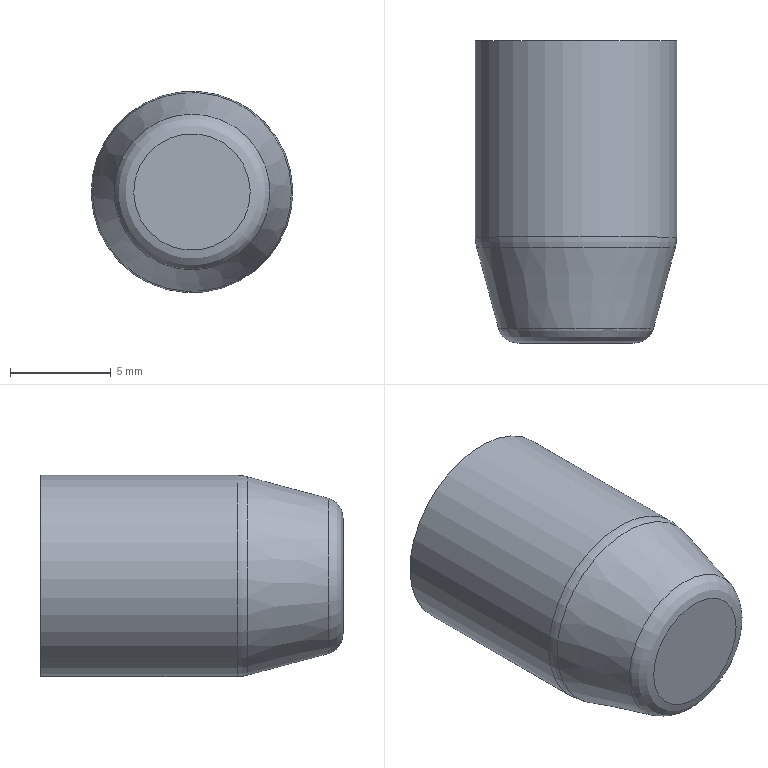Part | STEP file | 2_ESTAGIO_005 | 1 solid | 8 faces | box 10 x 15 x 10 mm | volume 994.545 mm3 | cone 2 | plane 2 | cylinder 2 | torus 2 | commonest cylinder face diameters 3.242 x1 10 x1
STEP:
#1=CARTESIAN_POINT('',(0.,0.,0.));
#2=DIRECTION('',(0.,0.,1.));
#3=DIRECTION('',(1.,0.,0.));
#4=AXIS2_PLACEMENT_3D('',#1,#2,#3);
#5=CARTESIAN_POINT('',(389.762,-538.65,378.626));
#6=VERTEX_POINT('',#5);
#7=CARTESIAN_POINT('',(388.339,-538.65,377.849));
#8=DIRECTION('',(0.,1.,0.));
#9=DIRECTION('',(1.,0.,0.));
#10=AXIS2_PLACEMENT_3D('',#7,#8,#9);
#11=CIRCLE('',#10,1.621);
#12=CARTESIAN_POINT('',(388.339,-539.009,377.849));
#13=DIRECTION('',(0.,1.,0.));
#14=DIRECTION('',(0.8776,0.,0.4794));
#15=AXIS2_PLACEMENT_3D('',#12,#13,#14);
#16=CONICAL_SURFACE('',#15,1.,1.047);
#17=CARTESIAN_POINT('',(-5.783,0.3585));
#18=DIRECTION('',(1.,0.));
#19=VECTOR('',#18,1.);
#20=LINE('',#17,#19);
#21=(GEOMETRIC_REPRESENTATION_CONTEXT(2)PARAMETRIC_REPRESENTATION_CONTEXT()REPRESENTATION_CONTEXT('',''));
#22=DEFINITIONAL_REPRESENTATION('',(#20),#21);
#23=PCURVE('',#16,#22);
#24=CARTESIAN_POINT('',(388.339,-528.75,377.849));
#25=DIRECTION('',(0.,-1.,0.));
#26=DIRECTION('',(0.8776,0.,0.4794));
#27=AXIS2_PLACEMENT_3D('',#24,#25,#26);
#28=CYLINDRICAL_SURFACE('',#27,1.621);
#29=CARTESIAN_POINT('',(12.066,9.9));
#30=DIRECTION('',(-1.,0.));
#31=VECTOR('',#30,1.);
#32=LINE('',#29,#31);
#33=(GEOMETRIC_REPRESENTATION_CONTEXT(2)PARAMETRIC_REPRESENTATION_CONTEXT()REPRESENTATION_CONTEXT('',''));
#34=DEFINITIONAL_REPRESENTATION('',(#32),#33);
#35=PCURVE('',#28,#34);
#36=SURFACE_CURVE('',#11,(#23,#35),.PCURVE_S1.);
#37=EDGE_CURVE('',#6,#6,#36,.T.);
#38=ORIENTED_EDGE('',*,*,#37,.F.);
#39=CARTESIAN_POINT('',(388.339,-539.586,377.849));
#40=VERTEX_POINT('',#39);
#41=CARTESIAN_POINT('',(388.339,-539.586,377.849));
#42=CARTESIAN_POINT('',(389.762,-538.65,378.626));
#43=B_SPLINE_CURVE_WITH_KNOTS('',1,(#41,#42),.UNSPECIFIED.,.F.,.F.,(2,2),(-1.155,0.7171),.PIECEWISE_BEZIER_KNOTS.);
#44=CARTESIAN_POINT('',(0.,0.));
#45=DIRECTION('',(0.,1.));
#46=VECTOR('',#45,1.);
#47=LINE('',#44,#46);
#48=(GEOMETRIC_REPRESENTATION_CONTEXT(2)PARAMETRIC_REPRESENTATION_CONTEXT()REPRESENTATION_CONTEXT('',''));
#49=DEFINITIONAL_REPRESENTATION('',(#47),#48);
#50=PCURVE('',#16,#49);
#51=CARTESIAN_POINT('',(6.283,0.));
#52=DIRECTION('',(0.,1.));
#53=VECTOR('',#52,1.);
#54=LINE('',#51,#53);
#55=(GEOMETRIC_REPRESENTATION_CONTEXT(2)PARAMETRIC_REPRESENTATION_CONTEXT()REPRESENTATION_CONTEXT('',''));
#56=DEFINITIONAL_REPRESENTATION('',(#54),#55);
#57=PCURVE('',#16,#56);
#58=SEAM_CURVE('',#43,(#50,#57),.PCURVE_S1.);
#59=EDGE_CURVE('',#40,#6,#58,.T.);
#60=ORIENTED_EDGE('',*,*,#59,.F.);
#61=ORIENTED_EDGE('',*,*,#59,.T.);
#62=EDGE_LOOP('',(#38,#60,#61));
#63=FACE_BOUND('',#62,.F.);
#64=ADVANCED_FACE('',(#63),#16,.F.);
#65=CARTESIAN_POINT('',(384.538,-528.65,381.097));
#66=VERTEX_POINT('',#65);
#67=CARTESIAN_POINT('',(388.339,-528.65,377.849));
#68=DIRECTION('',(0.,1.,0.));
#69=DIRECTION('',(1.,0.,0.));
#70=AXIS2_PLACEMENT_3D('',#67,#68,#69);
#71=CIRCLE('',#70,5.);
#72=CARTESIAN_POINT('',(393.232,-528.65,376.821));
#73=DIRECTION('',(0.,1.,0.));
#74=DIRECTION('',(0.,0.,1.));
#75=AXIS2_PLACEMENT_3D('',#72,#73,#74);
#76=PLANE('',#75);
#77=CARTESIAN_POINT('',(1.028,-4.893));
#78=DIRECTION('',(0.,1.));
#79=AXIS2_PLACEMENT_2D('',#77,#78);
#80=CIRCLE('',#79,5.);
#81=(GEOMETRIC_REPRESENTATION_CONTEXT(2)PARAMETRIC_REPRESENTATION_CONTEXT()REPRESENTATION_CONTEXT('',''));
#82=DEFINITIONAL_REPRESENTATION('',(#80),#81);
#83=PCURVE('',#76,#82);
#84=CARTESIAN_POINT('',(388.339,-536.15,377.849));
#85=DIRECTION('',(0.,1.,0.));
#86=DIRECTION('',(0.7602,0.,-0.6496));
#87=AXIS2_PLACEMENT_3D('',#84,#85,#86);
#88=CYLINDRICAL_SURFACE('',#87,5.);
#89=CARTESIAN_POINT('',(-0.7071,7.5));
#90=DIRECTION('',(1.,0.));
#91=VECTOR('',#90,1.);
#92=LINE('',#89,#91);
#93=(GEOMETRIC_REPRESENTATION_CONTEXT(2)PARAMETRIC_REPRESENTATION_CONTEXT()REPRESENTATION_CONTEXT('',''));
#94=DEFINITIONAL_REPRESENTATION('',(#92),#93);
#95=PCURVE('',#88,#94);
#96=SURFACE_CURVE('',#71,(#83,#95),.PCURVE_S1.);
#97=EDGE_CURVE('',#66,#66,#96,.T.);
#98=ORIENTED_EDGE('',*,*,#97,.T.);
#99=EDGE_LOOP('',(#98));
#100=FACE_BOUND('',#99,.T.);
#101=CARTESIAN_POINT('',(389.762,-528.65,378.626));
#102=VERTEX_POINT('',#101);
#103=CARTESIAN_POINT('',(388.339,-528.65,377.849));
#104=DIRECTION('',(0.,1.,0.));
#105=DIRECTION('',(1.,0.,0.));
#106=AXIS2_PLACEMENT_3D('',#103,#104,#105);
#107=CIRCLE('',#106,1.621);
#108=CARTESIAN_POINT('',(1.028,-4.893));
#109=DIRECTION('',(0.,1.));
#110=AXIS2_PLACEMENT_2D('',#108,#109);
#111=CIRCLE('',#110,1.621);
#112=(GEOMETRIC_REPRESENTATION_CONTEXT(2)PARAMETRIC_REPRESENTATION_CONTEXT()REPRESENTATION_CONTEXT('',''));
#113=DEFINITIONAL_REPRESENTATION('',(#111),#112);
#114=PCURVE('',#76,#113);
#115=CARTESIAN_POINT('',(12.066,-0.1));
#116=DIRECTION('',(-1.,0.));
#117=VECTOR('',#116,1.);
#118=LINE('',#115,#117);
#119=(GEOMETRIC_REPRESENTATION_CONTEXT(2)PARAMETRIC_REPRESENTATION_CONTEXT()REPRESENTATION_CONTEXT('',''));
#120=DEFINITIONAL_REPRESENTATION('',(#118),#119);
#121=PCURVE('',#28,#120);
#122=SURFACE_CURVE('',#107,(#114,#121),.PCURVE_S1.);
#123=EDGE_CURVE('',#102,#102,#122,.T.);
#124=ORIENTED_EDGE('',*,*,#123,.F.);
#125=EDGE_LOOP('',(#124));
#126=FACE_BOUND('',#125,.T.);
#127=ADVANCED_FACE('',(#100,#126),#76,.T.);
#128=CARTESIAN_POINT('',(384.538,-538.387,381.097));
#129=VERTEX_POINT('',#128);
#130=CARTESIAN_POINT('',(392.14,-538.387,374.601));
#131=VERTEX_POINT('',#130);
#132=CARTESIAN_POINT('',(388.339,-538.387,377.849));
#133=DIRECTION('',(0.,1.,0.));
#134=DIRECTION('',(1.,0.,0.));
#135=AXIS2_PLACEMENT_3D('',#132,#133,#134);
#136=CIRCLE('',#135,5.);
#137=CARTESIAN_POINT('',(-0.7071,-2.237));
#138=DIRECTION('',(1.,0.));
#139=VECTOR('',#138,1.);
#140=LINE('',#137,#139);
#141=(GEOMETRIC_REPRESENTATION_CONTEXT(2)PARAMETRIC_REPRESENTATION_CONTEXT()REPRESENTATION_CONTEXT('',''));
#142=DEFINITIONAL_REPRESENTATION('',(#140),#141);
#143=PCURVE('',#88,#142);
#144=CARTESIAN_POINT('',(388.339,-538.387,377.849));
#145=DIRECTION('',(0.,-1.,0.));
#146=DIRECTION('',(0.,0.,-1.));
#147=AXIS2_PLACEMENT_3D('',#144,#145,#146);
#148=TOROIDAL_SURFACE('',#147,3.,2.);
#149=CARTESIAN_POINT('',(7.854,6.283));
#150=DIRECTION('',(-1.,0.));
#151=VECTOR('',#150,1.);
#152=LINE('',#149,#151);
#153=(GEOMETRIC_REPRESENTATION_CONTEXT(2)PARAMETRIC_REPRESENTATION_CONTEXT()REPRESENTATION_CONTEXT('',''));
#154=DEFINITIONAL_REPRESENTATION('',(#152),#153);
#155=PCURVE('',#148,#154);
#156=SURFACE_CURVE('',#136,(#143,#155),.PCURVE_S1.);
#157=EDGE_CURVE('',#129,#131,#156,.T.);
#158=ORIENTED_EDGE('',*,*,#157,.T.);
#159=CARTESIAN_POINT('',(388.339,-538.387,377.849));
#160=DIRECTION('',(0.,1.,0.));
#161=DIRECTION('',(1.,0.,0.));
#162=AXIS2_PLACEMENT_3D('',#159,#160,#161);
#163=CIRCLE('',#162,5.);
#164=CARTESIAN_POINT('',(5.576,-2.237));
#165=DIRECTION('',(1.,0.));
#166=VECTOR('',#165,1.);
#167=LINE('',#164,#166);
#168=(GEOMETRIC_REPRESENTATION_CONTEXT(2)PARAMETRIC_REPRESENTATION_CONTEXT()REPRESENTATION_CONTEXT('',''));
#169=DEFINITIONAL_REPRESENTATION('',(#167),#168);
#170=PCURVE('',#88,#169);
#171=CARTESIAN_POINT('',(7.854,6.283));
#172=DIRECTION('',(-1.,0.));
#173=VECTOR('',#172,1.);
#174=LINE('',#171,#173);
#175=(GEOMETRIC_REPRESENTATION_CONTEXT(2)PARAMETRIC_REPRESENTATION_CONTEXT()REPRESENTATION_CONTEXT('',''));
#176=DEFINITIONAL_REPRESENTATION('',(#174),#175);
#177=PCURVE('',#148,#176);
#178=SURFACE_CURVE('',#163,(#170,#177),.PCURVE_S1.);
#179=EDGE_CURVE('',#131,#129,#178,.T.);
#180=ORIENTED_EDGE('',*,*,#179,.T.);
#181=CARTESIAN_POINT('',(384.538,-538.387,381.097));
#182=CARTESIAN_POINT('',(384.538,-528.65,381.097));
#183=B_SPLINE_CURVE_WITH_KNOTS('',1,(#181,#182),.UNSPECIFIED.,.F.,.F.,(2,2),(-2.237,7.5),.PIECEWISE_BEZIER_KNOTS.);
#184=CARTESIAN_POINT('',(9.425,0.));
#185=DIRECTION('',(0.,1.));
#186=VECTOR('',#185,1.);
#187=LINE('',#184,#186);
#188=(GEOMETRIC_REPRESENTATION_CONTEXT(2)PARAMETRIC_REPRESENTATION_CONTEXT()REPRESENTATION_CONTEXT('',''));
#189=DEFINITIONAL_REPRESENTATION('',(#187),#188);
#190=PCURVE('',#88,#189);
#191=CARTESIAN_POINT('',(3.142,0.));
#192=DIRECTION('',(0.,1.));
#193=VECTOR('',#192,1.);
#194=LINE('',#191,#193);
#195=(GEOMETRIC_REPRESENTATION_CONTEXT(2)PARAMETRIC_REPRESENTATION_CONTEXT()REPRESENTATION_CONTEXT('',''));
#196=DEFINITIONAL_REPRESENTATION('',(#194),#195);
#197=PCURVE('',#88,#196);
#198=SEAM_CURVE('',#183,(#190,#197),.PCURVE_S1.);
#199=EDGE_CURVE('',#129,#66,#198,.T.);
#200=ORIENTED_EDGE('',*,*,#199,.T.);
#201=ORIENTED_EDGE('',*,*,#97,.F.);
#202=ORIENTED_EDGE('',*,*,#199,.F.);
#203=EDGE_LOOP('',(#158,#180,#200,#201,#202));
#204=FACE_BOUND('',#203,.T.);
#205=ADVANCED_FACE('',(#204),#88,.T.);
#206=ORIENTED_EDGE('',*,*,#179,.F.);
#207=CARTESIAN_POINT('',(392.088,-538.904,374.645));
#208=VERTEX_POINT('',#207);
#209=CARTESIAN_POINT('',(392.14,-538.387,374.601));
#210=CARTESIAN_POINT('',(392.14,-538.474,374.601));
#211=CARTESIAN_POINT('',(392.137,-538.561,374.604));
#212=CARTESIAN_POINT('',(392.13,-538.648,374.61));
#213=CARTESIAN_POINT('',(392.119,-538.735,374.619));
#214=CARTESIAN_POINT('',(392.106,-538.82,374.631));
#215=CARTESIAN_POINT('',(392.088,-538.904,374.645));
#216=(BOUNDED_CURVE()B_SPLINE_CURVE(6,(#209,#210,#211,#212,#213,#214,#215),.UNSPECIFIED.,.F.,.F.)B_SPLINE_CURVE_WITH_KNOTS((7,7),(0.,0.2618),.PIECEWISE_BEZIER_KNOTS.)CURVE()GEOMETRIC_REPRESENTATION_ITEM()RATIONAL_B_SPLINE_CURVE((1.001,1.,0.9999,0.9998,0.9999,1.,1.001))REPRESENTATION_ITEM(''));
#217=CARTESIAN_POINT('',(7.147,6.283));
#218=DIRECTION('',(0.,1.));
#219=VECTOR('',#218,1.);
#220=LINE('',#217,#219);
#221=(GEOMETRIC_REPRESENTATION_CONTEXT(2)PARAMETRIC_REPRESENTATION_CONTEXT()REPRESENTATION_CONTEXT('',''));
#222=DEFINITIONAL_REPRESENTATION('',(#220),#221);
#223=PCURVE('',#148,#222);
#224=CARTESIAN_POINT('',(0.8637,6.283));
#225=DIRECTION('',(0.,1.));
#226=VECTOR('',#225,1.);
#227=LINE('',#224,#226);
#228=(GEOMETRIC_REPRESENTATION_CONTEXT(2)PARAMETRIC_REPRESENTATION_CONTEXT()REPRESENTATION_CONTEXT('',''));
#229=DEFINITIONAL_REPRESENTATION('',(#227),#228);
#230=PCURVE('',#148,#229);
#231=SEAM_CURVE('',#216,(#223,#230),.PCURVE_S1.);
#232=EDGE_CURVE('',#131,#208,#231,.T.);
#233=ORIENTED_EDGE('',*,*,#232,.T.);
#234=CARTESIAN_POINT('',(388.339,-538.904,377.849));
#235=DIRECTION('',(0.,-1.,0.));
#236=DIRECTION('',(1.,0.,0.));
#237=AXIS2_PLACEMENT_3D('',#234,#235,#236);
#238=CIRCLE('',#237,4.932);
#239=CARTESIAN_POINT('',(-4.712,6.545));
#240=DIRECTION('',(1.,0.));
#241=VECTOR('',#240,1.);
#242=LINE('',#239,#241);
#243=(GEOMETRIC_REPRESENTATION_CONTEXT(2)PARAMETRIC_REPRESENTATION_CONTEXT()REPRESENTATION_CONTEXT('',''));
#244=DEFINITIONAL_REPRESENTATION('',(#242),#243);
#245=PCURVE('',#148,#244);
#246=CARTESIAN_POINT('',(388.339,-543.65,377.849));
#247=DIRECTION('',(0.,1.,0.));
#248=DIRECTION('',(0.7602,0.,-0.6496));
#249=AXIS2_PLACEMENT_3D('',#246,#247,#248);
#250=CONICAL_SURFACE('',#249,3.66,0.2618);
#251=CARTESIAN_POINT('',(11.859,4.746));
#252=DIRECTION('',(-1.,0.));
#253=VECTOR('',#252,1.);
#254=LINE('',#251,#253);
#255=(GEOMETRIC_REPRESENTATION_CONTEXT(2)PARAMETRIC_REPRESENTATION_CONTEXT()REPRESENTATION_CONTEXT('',''));
#256=DEFINITIONAL_REPRESENTATION('',(#254),#255);
#257=PCURVE('',#250,#256);
#258=SURFACE_CURVE('',#238,(#245,#257),.PCURVE_S1.);
#259=EDGE_CURVE('',#208,#208,#258,.T.);
#260=ORIENTED_EDGE('',*,*,#259,.F.);
#261=ORIENTED_EDGE('',*,*,#232,.F.);
#262=ORIENTED_EDGE('',*,*,#157,.F.);
#263=EDGE_LOOP('',(#206,#233,#260,#261,#262));
#264=FACE_BOUND('',#263,.T.);
#265=ADVANCED_FACE('',(#264),#148,.T.);
#266=CARTESIAN_POINT('',(385.405,-542.909,380.356));
#267=VERTEX_POINT('',#266);
#268=CARTESIAN_POINT('',(391.273,-542.909,375.342));
#269=VERTEX_POINT('',#268);
#270=CARTESIAN_POINT('',(388.339,-542.909,377.849));
#271=DIRECTION('',(0.,1.,0.));
#272=DIRECTION('',(1.,0.,0.));
#273=AXIS2_PLACEMENT_3D('',#270,#271,#272);
#274=CIRCLE('',#273,3.859);
#275=CARTESIAN_POINT('',(-0.7071,0.7412));
#276=DIRECTION('',(1.,0.));
#277=VECTOR('',#276,1.);
#278=LINE('',#275,#277);
#279=(GEOMETRIC_REPRESENTATION_CONTEXT(2)PARAMETRIC_REPRESENTATION_CONTEXT()REPRESENTATION_CONTEXT('',''));
#280=DEFINITIONAL_REPRESENTATION('',(#278),#279);
#281=PCURVE('',#250,#280);
#282=CARTESIAN_POINT('',(388.339,-542.65,377.849));
#283=DIRECTION('',(0.,1.,0.));
#284=DIRECTION('',(0.,0.,1.));
#285=AXIS2_PLACEMENT_3D('',#282,#283,#284);
#286=TOROIDAL_SURFACE('',#285,2.893,1.);
#287=CARTESIAN_POINT('',(1.571,6.021));
#288=DIRECTION('',(1.,0.));
#289=VECTOR('',#288,1.);
#290=LINE('',#287,#289);
#291=(GEOMETRIC_REPRESENTATION_CONTEXT(2)PARAMETRIC_REPRESENTATION_CONTEXT()REPRESENTATION_CONTEXT('',''));
#292=DEFINITIONAL_REPRESENTATION('',(#290),#291);
#293=PCURVE('',#286,#292);
#294=SURFACE_CURVE('',#274,(#281,#293),.PCURVE_S1.);
#295=EDGE_CURVE('',#267,#269,#294,.T.);
#296=ORIENTED_EDGE('',*,*,#295,.T.);
#297=CARTESIAN_POINT('',(391.273,-542.909,375.342));
#298=CARTESIAN_POINT('',(392.088,-538.904,374.645));
#299=B_SPLINE_CURVE_WITH_KNOTS('',1,(#297,#298),.UNSPECIFIED.,.F.,.F.,(2,2),(0.7673,4.913),.PIECEWISE_BEZIER_KNOTS.);
#300=CARTESIAN_POINT('',(6.283,0.));
#301=DIRECTION('',(0.,1.));
#302=VECTOR('',#301,1.);
#303=LINE('',#300,#302);
#304=(GEOMETRIC_REPRESENTATION_CONTEXT(2)PARAMETRIC_REPRESENTATION_CONTEXT()REPRESENTATION_CONTEXT('',''));
#305=DEFINITIONAL_REPRESENTATION('',(#303),#304);
#306=PCURVE('',#250,#305);
#307=CARTESIAN_POINT('',(0.,0.));
#308=DIRECTION('',(0.,1.));
#309=VECTOR('',#308,1.);
#310=LINE('',#307,#309);
#311=(GEOMETRIC_REPRESENTATION_CONTEXT(2)PARAMETRIC_REPRESENTATION_CONTEXT()REPRESENTATION_CONTEXT('',''));
#312=DEFINITIONAL_REPRESENTATION('',(#310),#311);
#313=PCURVE('',#250,#312);
#314=SEAM_CURVE('',#299,(#306,#313),.PCURVE_S1.);
#315=EDGE_CURVE('',#269,#208,#314,.T.);
#316=ORIENTED_EDGE('',*,*,#315,.T.);
#317=ORIENTED_EDGE('',*,*,#259,.T.);
#318=ORIENTED_EDGE('',*,*,#315,.F.);
#319=CARTESIAN_POINT('',(388.339,-542.909,377.849));
#320=DIRECTION('',(0.,1.,0.));
#321=DIRECTION('',(1.,0.,0.));
#322=AXIS2_PLACEMENT_3D('',#319,#320,#321);
#323=CIRCLE('',#322,3.859);
#324=CARTESIAN_POINT('',(-0.7071,0.7412));
#325=DIRECTION('',(1.,0.));
#326=VECTOR('',#325,1.);
#327=LINE('',#324,#326);
#328=(GEOMETRIC_REPRESENTATION_CONTEXT(2)PARAMETRIC_REPRESENTATION_CONTEXT()REPRESENTATION_CONTEXT('',''));
#329=DEFINITIONAL_REPRESENTATION('',(#327),#328);
#330=PCURVE('',#250,#329);
#331=CARTESIAN_POINT('',(1.571,6.021));
#332=DIRECTION('',(1.,0.));
#333=VECTOR('',#332,1.);
#334=LINE('',#331,#333);
#335=(GEOMETRIC_REPRESENTATION_CONTEXT(2)PARAMETRIC_REPRESENTATION_CONTEXT()REPRESENTATION_CONTEXT('',''));
#336=DEFINITIONAL_REPRESENTATION('',(#334),#335);
#337=PCURVE('',#286,#336);
#338=SURFACE_CURVE('',#323,(#330,#337),.PCURVE_S1.);
#339=EDGE_CURVE('',#269,#267,#338,.T.);
#340=ORIENTED_EDGE('',*,*,#339,.T.);
#341=EDGE_LOOP('',(#296,#316,#317,#318,#340));
#342=FACE_BOUND('',#341,.T.);
#343=ADVANCED_FACE('',(#342),#250,.T.);
#344=ORIENTED_EDGE('',*,*,#295,.F.);
#345=ORIENTED_EDGE('',*,*,#339,.F.);
#346=CARTESIAN_POINT('',(390.538,-543.65,375.97));
#347=VERTEX_POINT('',#346);
#348=CARTESIAN_POINT('',(390.538,-543.65,375.97));
#349=CARTESIAN_POINT('',(390.707,-543.65,375.826));
#350=CARTESIAN_POINT('',(390.872,-543.592,375.685));
#351=CARTESIAN_POINT('',(391.021,-543.478,375.557));
#352=CARTESIAN_POINT('',(391.143,-543.317,375.453));
#353=CARTESIAN_POINT('',(391.229,-543.123,375.38));
#354=CARTESIAN_POINT('',(391.273,-542.909,375.342));
#355=(BOUNDED_CURVE()B_SPLINE_CURVE(6,(#348,#349,#350,#351,#352,#353,#354),.UNSPECIFIED.,.F.,.F.)B_SPLINE_CURVE_WITH_KNOTS((7,7),(4.712,6.021),.PIECEWISE_BEZIER_KNOTS.)CURVE()GEOMETRIC_REPRESENTATION_ITEM()RATIONAL_B_SPLINE_CURVE((1.022,1.007,0.9986,0.9958,0.9986,1.007,1.022))REPRESENTATION_ITEM(''));
#356=CARTESIAN_POINT('',(2.278,0.));
#357=DIRECTION('',(0.,1.));
#358=VECTOR('',#357,1.);
#359=LINE('',#356,#358);
#360=(GEOMETRIC_REPRESENTATION_CONTEXT(2)PARAMETRIC_REPRESENTATION_CONTEXT()REPRESENTATION_CONTEXT('',''));
#361=DEFINITIONAL_REPRESENTATION('',(#359),#360);
#362=PCURVE('',#286,#361);
#363=CARTESIAN_POINT('',(8.561,0.));
#364=DIRECTION('',(0.,1.));
#365=VECTOR('',#364,1.);
#366=LINE('',#363,#365);
#367=(GEOMETRIC_REPRESENTATION_CONTEXT(2)PARAMETRIC_REPRESENTATION_CONTEXT()REPRESENTATION_CONTEXT('',''));
#368=DEFINITIONAL_REPRESENTATION('',(#366),#367);
#369=PCURVE('',#286,#368);
#370=SEAM_CURVE('',#355,(#362,#369),.PCURVE_S1.);
#371=EDGE_CURVE('',#347,#269,#370,.T.);
#372=ORIENTED_EDGE('',*,*,#371,.F.);
#373=CARTESIAN_POINT('',(388.339,-543.65,377.849));
#374=DIRECTION('',(0.,1.,0.));
#375=DIRECTION('',(1.,0.,0.));
#376=AXIS2_PLACEMENT_3D('',#373,#374,#375);
#377=CIRCLE('',#376,2.893);
#378=CARTESIAN_POINT('',(1.571,4.712));
#379=DIRECTION('',(1.,0.));
#380=VECTOR('',#379,1.);
#381=LINE('',#378,#380);
#382=(GEOMETRIC_REPRESENTATION_CONTEXT(2)PARAMETRIC_REPRESENTATION_CONTEXT()REPRESENTATION_CONTEXT('',''));
#383=DEFINITIONAL_REPRESENTATION('',(#381),#382);
#384=PCURVE('',#286,#383);
#385=CARTESIAN_POINT('',(388.339,-543.65,377.849));
#386=DIRECTION('',(0.,1.,0.));
#387=DIRECTION('',(0.,0.,1.));
#388=AXIS2_PLACEMENT_3D('',#385,#386,#387);
#389=PLANE('',#388);
#390=CARTESIAN_POINT('',(0.,0.));
#391=DIRECTION('',(0.,1.));
#392=AXIS2_PLACEMENT_2D('',#390,#391);
#393=CIRCLE('',#392,2.893);
#394=(GEOMETRIC_REPRESENTATION_CONTEXT(2)PARAMETRIC_REPRESENTATION_CONTEXT()REPRESENTATION_CONTEXT('',''));
#395=DEFINITIONAL_REPRESENTATION('',(#393),#394);
#396=PCURVE('',#389,#395);
#397=SURFACE_CURVE('',#377,(#384,#396),.PCURVE_S1.);
#398=EDGE_CURVE('',#347,#347,#397,.T.);
#399=ORIENTED_EDGE('',*,*,#398,.T.);
#400=ORIENTED_EDGE('',*,*,#371,.T.);
#401=EDGE_LOOP('',(#344,#345,#372,#399,#400));
#402=FACE_BOUND('',#401,.T.);
#403=ADVANCED_FACE('',(#402),#286,.T.);
#404=ORIENTED_EDGE('',*,*,#398,.F.);
#405=EDGE_LOOP('',(#404));
#406=FACE_BOUND('',#405,.T.);
#407=ADVANCED_FACE('',(#406),#389,.F.);
#408=ORIENTED_EDGE('',*,*,#123,.F.);
#409=CARTESIAN_POINT('',(389.762,-528.65,378.626));
#410=CARTESIAN_POINT('',(389.762,-538.65,378.626));
#411=B_SPLINE_CURVE_WITH_KNOTS('',1,(#409,#410),.UNSPECIFIED.,.F.,.F.,(2,2),(-0.1,9.9),.PIECEWISE_BEZIER_KNOTS.);
#412=CARTESIAN_POINT('',(6.283,0.));
#413=DIRECTION('',(0.,1.));
#414=VECTOR('',#413,1.);
#415=LINE('',#412,#414);
#416=(GEOMETRIC_REPRESENTATION_CONTEXT(2)PARAMETRIC_REPRESENTATION_CONTEXT()REPRESENTATION_CONTEXT('',''));
#417=DEFINITIONAL_REPRESENTATION('',(#415),#416);
#418=PCURVE('',#28,#417);
#419=CARTESIAN_POINT('',(0.,0.));
#420=DIRECTION('',(0.,1.));
#421=VECTOR('',#420,1.);
#422=LINE('',#419,#421);
#423=(GEOMETRIC_REPRESENTATION_CONTEXT(2)PARAMETRIC_REPRESENTATION_CONTEXT()REPRESENTATION_CONTEXT('',''));
#424=DEFINITIONAL_REPRESENTATION('',(#422),#423);
#425=PCURVE('',#28,#424);
#426=SEAM_CURVE('',#411,(#418,#425),.PCURVE_S1.);
#427=EDGE_CURVE('',#102,#6,#426,.T.);
#428=ORIENTED_EDGE('',*,*,#427,.T.);
#429=ORIENTED_EDGE('',*,*,#37,.T.);
#430=ORIENTED_EDGE('',*,*,#427,.F.);
#431=EDGE_LOOP('',(#408,#428,#429,#430));
#432=FACE_BOUND('',#431,.F.);
#433=ADVANCED_FACE('',(#432),#28,.F.);
#434=CLOSED_SHELL('',(#64,#127,#205,#265,#343,#403,#407,#433));
#435=MANIFOLD_SOLID_BREP('',#434);
#436=(LENGTH_UNIT()NAMED_UNIT(*)SI_UNIT(.MILLI.,.METRE.));
#437=UNCERTAINTY_MEASURE_WITH_UNIT(LENGTH_MEASURE(0.00001),#436,'','');
#438=(NAMED_UNIT(*)PLANE_ANGLE_UNIT()SI_UNIT($,.RADIAN.));
#439=(NAMED_UNIT(*)SI_UNIT($,.STERADIAN.)SOLID_ANGLE_UNIT());
#440=(GEOMETRIC_REPRESENTATION_CONTEXT(3)GLOBAL_UNCERTAINTY_ASSIGNED_CONTEXT((#437))GLOBAL_UNIT_ASSIGNED_CONTEXT((#436,#438,#439))REPRESENTATION_CONTEXT('',''));
#441=ADVANCED_BREP_SHAPE_REPRESENTATION('',(#4,#435),#440);